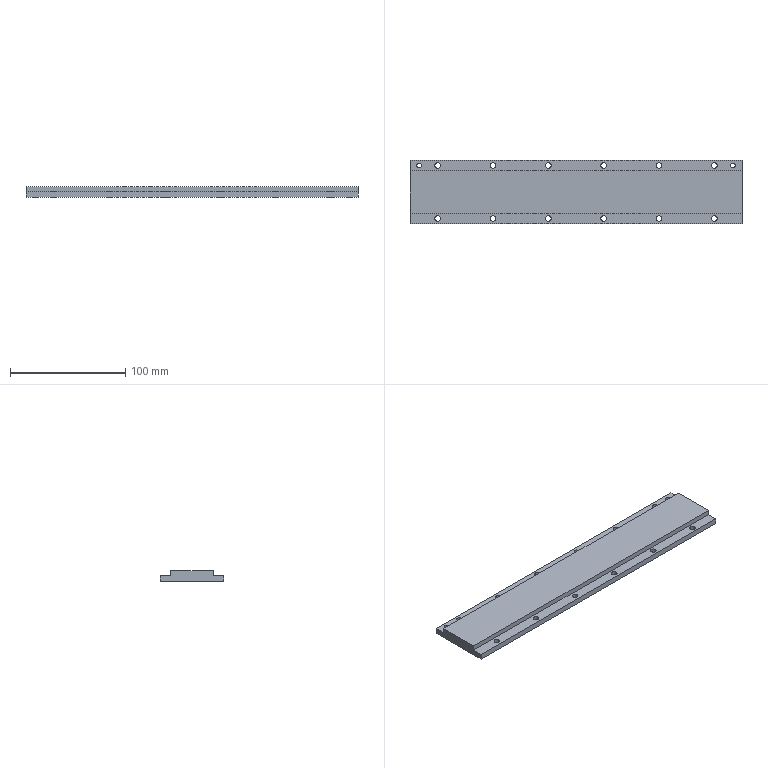Part | STEP file | 1 solid | 38 faces | box 288 x 55 x 9.4 mm | volume 124869 mm3 | cylinder 28 | plane 10 | commonest cylinder face diameters 4.8 x24 4.1 x4